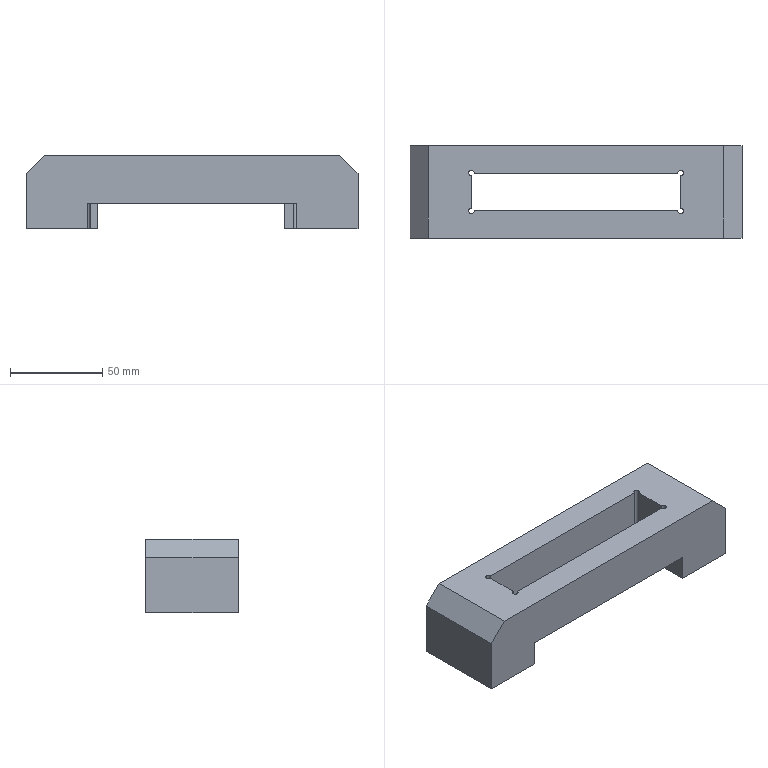Part | SolidWorks | features ICE 3, Chamfer 1, Cut 1, Extrusion 1 | 1 solid | 25 faces | box 180 x 50 x 40 mm | volume 216729 mm3 | plane 19 | cylinder 6 | commonest cylinder face diameters 3 x6
STEP:
#1=CARTESIAN_POINT('',(58.25,-10.25,0.));
#2=VERTEX_POINT('',#1);
#3=CARTESIAN_POINT('',(56.75,-8.75,0.));
#4=VERTEX_POINT('',#3);
#5=CARTESIAN_POINT('',(56.75,-10.25,0.));
#6=DIRECTION('',(0.,0.,1.));
#7=DIRECTION('',(1.,0.,0.));
#8=AXIS2_PLACEMENT_3D('',#5,#6,#7);
#9=CIRCLE('',#8,1.5);
#10=EDGE_CURVE('',#2,#4,#9,.T.);
#11=ORIENTED_EDGE('',*,*,#10,.F.);
#12=CARTESIAN_POINT('',(58.25,-10.25,40.));
#13=VERTEX_POINT('',#12);
#14=CARTESIAN_POINT('',(58.25,-10.25,0.));
#15=DIRECTION('',(0.,0.,1.));
#16=VECTOR('',#15,1000.);
#17=LINE('',#14,#16);
#18=EDGE_CURVE('',#2,#13,#17,.T.);
#19=ORIENTED_EDGE('',*,*,#18,.T.);
#20=CARTESIAN_POINT('',(56.75,-8.75,40.));
#21=VERTEX_POINT('',#20);
#22=CARTESIAN_POINT('',(56.75,-10.25,40.));
#23=DIRECTION('',(0.,0.,1.));
#24=DIRECTION('',(1.,0.,0.));
#25=AXIS2_PLACEMENT_3D('',#22,#23,#24);
#26=CIRCLE('',#25,1.5);
#27=EDGE_CURVE('',#13,#21,#26,.T.);
#28=ORIENTED_EDGE('',*,*,#27,.T.);
#29=CARTESIAN_POINT('',(56.75,-8.75,0.));
#30=DIRECTION('',(0.,0.,1.));
#31=VECTOR('',#30,1000.);
#32=LINE('',#29,#31);
#33=EDGE_CURVE('',#4,#21,#32,.T.);
#34=ORIENTED_EDGE('',*,*,#33,.F.);
#35=EDGE_LOOP('',(#11,#19,#28,#34));
#36=FACE_OUTER_BOUND('',#35,.T.);
#37=CARTESIAN_POINT('',(56.75,-10.25,0.));
#38=DIRECTION('',(0.,0.,1.));
#39=DIRECTION('',(1.,0.,0.));
#40=AXIS2_PLACEMENT_3D('',#37,#38,#39);
#41=CYLINDRICAL_SURFACE('',#40,1.5);
#42=ADVANCED_FACE('',(#36),#41,.F.);
#43=CARTESIAN_POINT('',(58.25,10.25,0.));
#44=VERTEX_POINT('',#43);
#45=CARTESIAN_POINT('',(55.25,10.25,0.));
#46=VERTEX_POINT('',#45);
#47=CARTESIAN_POINT('',(56.75,10.25,0.));
#48=DIRECTION('',(0.,0.,1.));
#49=DIRECTION('',(1.,0.,0.));
#50=AXIS2_PLACEMENT_3D('',#47,#48,#49);
#51=CIRCLE('',#50,1.5);
#52=EDGE_CURVE('',#44,#46,#51,.T.);
#53=ORIENTED_EDGE('',*,*,#52,.F.);
#54=CARTESIAN_POINT('',(58.25,10.25,40.));
#55=VERTEX_POINT('',#54);
#56=CARTESIAN_POINT('',(58.25,10.25,0.));
#57=DIRECTION('',(0.,0.,1.));
#58=VECTOR('',#57,1000.);
#59=LINE('',#56,#58);
#60=EDGE_CURVE('',#44,#55,#59,.T.);
#61=ORIENTED_EDGE('',*,*,#60,.T.);
#62=CARTESIAN_POINT('',(55.25,10.25,40.));
#63=VERTEX_POINT('',#62);
#64=CARTESIAN_POINT('',(56.75,10.25,40.));
#65=DIRECTION('',(0.,0.,1.));
#66=DIRECTION('',(1.,0.,0.));
#67=AXIS2_PLACEMENT_3D('',#64,#65,#66);
#68=CIRCLE('',#67,1.5);
#69=EDGE_CURVE('',#55,#63,#68,.T.);
#70=ORIENTED_EDGE('',*,*,#69,.T.);
#71=CARTESIAN_POINT('',(55.25,10.25,0.));
#72=DIRECTION('',(0.,0.,1.));
#73=VECTOR('',#72,1000.);
#74=LINE('',#71,#73);
#75=EDGE_CURVE('',#46,#63,#74,.T.);
#76=ORIENTED_EDGE('',*,*,#75,.F.);
#77=EDGE_LOOP('',(#53,#61,#70,#76));
#78=FACE_OUTER_BOUND('',#77,.T.);
#79=CARTESIAN_POINT('',(56.75,10.25,0.));
#80=DIRECTION('',(0.,0.,1.));
#81=DIRECTION('',(1.,0.,0.));
#82=AXIS2_PLACEMENT_3D('',#79,#80,#81);
#83=CYLINDRICAL_SURFACE('',#82,1.5);
#84=ADVANCED_FACE('',(#78),#83,.F.);
#85=CARTESIAN_POINT('',(-56.75,-8.75,0.));
#86=VERTEX_POINT('',#85);
#87=CARTESIAN_POINT('',(-56.75,-11.75,0.));
#88=VERTEX_POINT('',#87);
#89=CARTESIAN_POINT('',(-56.75,-10.25,0.));
#90=DIRECTION('',(0.,0.,1.));
#91=DIRECTION('',(1.,0.,0.));
#92=AXIS2_PLACEMENT_3D('',#89,#90,#91);
#93=CIRCLE('',#92,1.5);
#94=EDGE_CURVE('',#86,#88,#93,.T.);
#95=ORIENTED_EDGE('',*,*,#94,.T.);
#96=CARTESIAN_POINT('',(-56.75,-25.,0.));
#97=VERTEX_POINT('',#96);
#98=CARTESIAN_POINT('',(-56.75,-25.,0.));
#99=DIRECTION('',(0.,1.,0.));
#100=VECTOR('',#99,1000.);
#101=LINE('',#98,#100);
#102=EDGE_CURVE('',#97,#88,#101,.T.);
#103=ORIENTED_EDGE('',*,*,#102,.F.);
#104=CARTESIAN_POINT('',(-90.,-25.,0.));
#105=VERTEX_POINT('',#104);
#106=CARTESIAN_POINT('',(-90.,-25.,0.));
#107=DIRECTION('',(1.,0.,0.));
#108=VECTOR('',#107,1000.);
#109=LINE('',#106,#108);
#110=EDGE_CURVE('',#105,#97,#109,.T.);
#111=ORIENTED_EDGE('',*,*,#110,.F.);
#112=CARTESIAN_POINT('',(-90.,25.,0.));
#113=VERTEX_POINT('',#112);
#114=CARTESIAN_POINT('',(-90.,25.,0.));
#115=DIRECTION('',(0.,-1.,0.));
#116=VECTOR('',#115,1000.);
#117=LINE('',#114,#116);
#118=EDGE_CURVE('',#113,#105,#117,.T.);
#119=ORIENTED_EDGE('',*,*,#118,.F.);
#120=CARTESIAN_POINT('',(-51.16,25.,0.));
#121=VERTEX_POINT('',#120);
#122=CARTESIAN_POINT('',(-90.,25.,0.));
#123=DIRECTION('',(-1.,0.,0.));
#124=VECTOR('',#123,1000.);
#125=LINE('',#122,#124);
#126=EDGE_CURVE('',#121,#113,#125,.T.);
#127=ORIENTED_EDGE('',*,*,#126,.F.);
#128=CARTESIAN_POINT('',(-51.16,10.25,0.));
#129=VERTEX_POINT('',#128);
#130=CARTESIAN_POINT('',(-51.16,-5.,0.));
#131=DIRECTION('',(0.,1.,0.));
#132=VECTOR('',#131,1000.);
#133=LINE('',#130,#132);
#134=EDGE_CURVE('',#129,#121,#133,.T.);
#135=ORIENTED_EDGE('',*,*,#134,.F.);
#136=CARTESIAN_POINT('',(-55.25,10.25,0.));
#137=VERTEX_POINT('',#136);
#138=CARTESIAN_POINT('',(-56.75,10.25,0.));
#139=DIRECTION('',(-1.,0.,0.));
#140=VECTOR('',#139,1000.);
#141=LINE('',#138,#140);
#142=EDGE_CURVE('',#129,#137,#141,.T.);
#143=ORIENTED_EDGE('',*,*,#142,.T.);
#144=CARTESIAN_POINT('',(-56.75,8.75,0.));
#145=VERTEX_POINT('',#144);
#146=CARTESIAN_POINT('',(-56.75,10.25,0.));
#147=DIRECTION('',(0.,0.,1.));
#148=DIRECTION('',(1.,0.,0.));
#149=AXIS2_PLACEMENT_3D('',#146,#147,#148);
#150=CIRCLE('',#149,1.5);
#151=EDGE_CURVE('',#137,#145,#150,.T.);
#152=ORIENTED_EDGE('',*,*,#151,.T.);
#153=CARTESIAN_POINT('',(-56.75,10.25,0.));
#154=DIRECTION('',(0.,-1.,0.));
#155=VECTOR('',#154,1000.);
#156=LINE('',#153,#155);
#157=EDGE_CURVE('',#145,#86,#156,.T.);
#158=ORIENTED_EDGE('',*,*,#157,.T.);
#159=EDGE_LOOP('',(#95,#103,#111,#119,#127,#135,#143,#152,#158));
#160=FACE_OUTER_BOUND('',#159,.T.);
#161=CARTESIAN_POINT('',(0.,0.,0.));
#162=DIRECTION('',(0.,0.,1.));
#163=DIRECTION('',(1.,0.,0.));
#164=AXIS2_PLACEMENT_3D('',#161,#162,#163);
#165=PLANE('',#164);
#166=ADVANCED_FACE('',(#160),#165,.F.);
#167=CARTESIAN_POINT('',(-55.25,-10.25,14.));
#168=VERTEX_POINT('',#167);
#169=CARTESIAN_POINT('',(55.25,-10.25,14.));
#170=VERTEX_POINT('',#169);
#171=CARTESIAN_POINT('',(-56.75,-10.25,14.));
#172=DIRECTION('',(1.,0.,0.));
#173=VECTOR('',#172,1000.);
#174=LINE('',#171,#173);
#175=EDGE_CURVE('',#168,#170,#174,.T.);
#176=ORIENTED_EDGE('',*,*,#175,.F.);
#177=CARTESIAN_POINT('',(-55.25,-10.25,40.));
#178=VERTEX_POINT('',#177);
#179=CARTESIAN_POINT('',(-55.25,-10.25,0.));
#180=DIRECTION('',(0.,0.,1.));
#181=VECTOR('',#180,1000.);
#182=LINE('',#179,#181);
#183=EDGE_CURVE('',#168,#178,#182,.T.);
#184=ORIENTED_EDGE('',*,*,#183,.T.);
#185=CARTESIAN_POINT('',(55.25,-10.25,40.));
#186=VERTEX_POINT('',#185);
#187=CARTESIAN_POINT('',(-56.75,-10.25,40.));
#188=DIRECTION('',(1.,0.,0.));
#189=VECTOR('',#188,1000.);
#190=LINE('',#187,#189);
#191=EDGE_CURVE('',#178,#186,#190,.T.);
#192=ORIENTED_EDGE('',*,*,#191,.T.);
#193=CARTESIAN_POINT('',(55.25,-10.25,0.));
#194=DIRECTION('',(0.,0.,-1.));
#195=VECTOR('',#194,1000.);
#196=LINE('',#193,#195);
#197=EDGE_CURVE('',#186,#170,#196,.T.);
#198=ORIENTED_EDGE('',*,*,#197,.T.);
#199=EDGE_LOOP('',(#176,#184,#192,#198));
#200=FACE_OUTER_BOUND('',#199,.T.);
#201=CARTESIAN_POINT('',(-56.75,-10.25,0.));
#202=DIRECTION('',(0.,-1.,0.));
#203=DIRECTION('',(0.,0.,-1.));
#204=AXIS2_PLACEMENT_3D('',#201,#202,#203);
#205=PLANE('',#204);
#206=ADVANCED_FACE('',(#200),#205,.F.);
#207=CARTESIAN_POINT('',(-90.,-25.,30.));
#208=VERTEX_POINT('',#207);
#209=CARTESIAN_POINT('',(-90.,-25.,40.));
#210=DIRECTION('',(0.,0.,-1.));
#211=VECTOR('',#210,1000.);
#212=LINE('',#209,#211);
#213=EDGE_CURVE('',#208,#105,#212,.T.);
#214=ORIENTED_EDGE('',*,*,#213,.F.);
#215=CARTESIAN_POINT('',(-90.,25.,30.));
#216=VERTEX_POINT('',#215);
#217=CARTESIAN_POINT('',(-90.,25.,30.));
#218=DIRECTION('',(0.,1.,0.));
#219=VECTOR('',#218,1000.);
#220=LINE('',#217,#219);
#221=EDGE_CURVE('',#208,#216,#220,.T.);
#222=ORIENTED_EDGE('',*,*,#221,.T.);
#223=CARTESIAN_POINT('',(-90.,25.,40.));
#224=DIRECTION('',(0.,0.,-1.));
#225=VECTOR('',#224,1000.);
#226=LINE('',#223,#225);
#227=EDGE_CURVE('',#216,#113,#226,.T.);
#228=ORIENTED_EDGE('',*,*,#227,.T.);
#229=ORIENTED_EDGE('',*,*,#118,.T.);
#230=EDGE_LOOP('',(#214,#222,#228,#229));
#231=FACE_OUTER_BOUND('',#230,.T.);
#232=CARTESIAN_POINT('',(-90.,25.,40.));
#233=DIRECTION('',(1.,0.,0.));
#234=DIRECTION('',(0.,0.,-1.));
#235=AXIS2_PLACEMENT_3D('',#232,#233,#234);
#236=PLANE('',#235);
#237=ADVANCED_FACE('',(#231),#236,.F.);
#238=CARTESIAN_POINT('',(-80.,-25.,40.));
#239=VERTEX_POINT('',#238);
#240=CARTESIAN_POINT('',(80.,-25.,40.));
#241=VERTEX_POINT('',#240);
#242=CARTESIAN_POINT('',(-90.,-25.,40.));
#243=DIRECTION('',(1.,0.,0.));
#244=VECTOR('',#243,1000.);
#245=LINE('',#242,#244);
#246=EDGE_CURVE('',#239,#241,#245,.T.);
#247=ORIENTED_EDGE('',*,*,#246,.F.);
#248=CARTESIAN_POINT('',(-80.,-25.,40.));
#249=DIRECTION('',(-0.7071,0.,-0.7071));
#250=VECTOR('',#249,1000.);
#251=LINE('',#248,#250);
#252=EDGE_CURVE('',#239,#208,#251,.T.);
#253=ORIENTED_EDGE('',*,*,#252,.T.);
#254=ORIENTED_EDGE('',*,*,#213,.T.);
#255=ORIENTED_EDGE('',*,*,#110,.T.);
#256=CARTESIAN_POINT('',(-56.75,-25.,14.));
#257=VERTEX_POINT('',#256);
#258=CARTESIAN_POINT('',(-56.75,-25.,14.));
#259=DIRECTION('',(0.,0.,-1.));
#260=VECTOR('',#259,1000.);
#261=LINE('',#258,#260);
#262=EDGE_CURVE('',#257,#97,#261,.T.);
#263=ORIENTED_EDGE('',*,*,#262,.F.);
#264=CARTESIAN_POINT('',(56.75,-25.,14.));
#265=VERTEX_POINT('',#264);
#266=CARTESIAN_POINT('',(-56.75,-25.,14.));
#267=DIRECTION('',(-1.,0.,0.));
#268=VECTOR('',#267,1000.);
#269=LINE('',#266,#268);
#270=EDGE_CURVE('',#265,#257,#269,.T.);
#271=ORIENTED_EDGE('',*,*,#270,.F.);
#272=CARTESIAN_POINT('',(56.75,-25.,0.));
#273=VERTEX_POINT('',#272);
#274=CARTESIAN_POINT('',(56.75,-25.,14.));
#275=DIRECTION('',(0.,0.,-1.));
#276=VECTOR('',#275,1000.);
#277=LINE('',#274,#276);
#278=EDGE_CURVE('',#265,#273,#277,.T.);
#279=ORIENTED_EDGE('',*,*,#278,.T.);
#280=CARTESIAN_POINT('',(90.,-25.,0.));
#281=VERTEX_POINT('',#280);
#282=CARTESIAN_POINT('',(-90.,-25.,0.));
#283=DIRECTION('',(1.,0.,0.));
#284=VECTOR('',#283,1000.);
#285=LINE('',#282,#284);
#286=EDGE_CURVE('',#273,#281,#285,.T.);
#287=ORIENTED_EDGE('',*,*,#286,.T.);
#288=CARTESIAN_POINT('',(90.,-25.,30.));
#289=VERTEX_POINT('',#288);
#290=CARTESIAN_POINT('',(90.,-25.,40.));
#291=DIRECTION('',(0.,0.,-1.));
#292=VECTOR('',#291,1000.);
#293=LINE('',#290,#292);
#294=EDGE_CURVE('',#289,#281,#293,.T.);
#295=ORIENTED_EDGE('',*,*,#294,.F.);
#296=CARTESIAN_POINT('',(80.,-25.,40.));
#297=DIRECTION('',(-0.7071,0.,0.7071));
#298=VECTOR('',#297,1000.);
#299=LINE('',#296,#298);
#300=EDGE_CURVE('',#289,#241,#299,.T.);
#301=ORIENTED_EDGE('',*,*,#300,.T.);
#302=EDGE_LOOP('',(#247,#253,#254,#255,#263,#271,#279,#287,#295,#301));
#303=FACE_OUTER_BOUND('',#302,.T.);
#304=CARTESIAN_POINT('',(-90.,-25.,40.));
#305=DIRECTION('',(0.,1.,0.));
#306=DIRECTION('',(0.,0.,1.));
#307=AXIS2_PLACEMENT_3D('',#304,#305,#306);
#308=PLANE('',#307);
#309=ADVANCED_FACE('',(#303),#308,.F.);
#310=CARTESIAN_POINT('',(90.,25.,30.));
#311=VERTEX_POINT('',#310);
#312=CARTESIAN_POINT('',(90.,25.,0.));
#313=VERTEX_POINT('',#312);
#314=CARTESIAN_POINT('',(90.,25.,40.));
#315=DIRECTION('',(0.,0.,-1.));
#316=VECTOR('',#315,1000.);
#317=LINE('',#314,#316);
#318=EDGE_CURVE('',#311,#313,#317,.T.);
#319=ORIENTED_EDGE('',*,*,#318,.F.);
#320=CARTESIAN_POINT('',(90.,-25.,30.));
#321=DIRECTION('',(0.,-1.,0.));
#322=VECTOR('',#321,1000.);
#323=LINE('',#320,#322);
#324=EDGE_CURVE('',#311,#289,#323,.T.);
#325=ORIENTED_EDGE('',*,*,#324,.T.);
#326=ORIENTED_EDGE('',*,*,#294,.T.);
#327=CARTESIAN_POINT('',(90.,25.,0.));
#328=DIRECTION('',(0.,1.,0.));
#329=VECTOR('',#328,1000.);
#330=LINE('',#327,#329);
#331=EDGE_CURVE('',#281,#313,#330,.T.);
#332=ORIENTED_EDGE('',*,*,#331,.T.);
#333=EDGE_LOOP('',(#319,#325,#326,#332));
#334=FACE_OUTER_BOUND('',#333,.T.);
#335=CARTESIAN_POINT('',(90.,25.,40.));
#336=DIRECTION('',(-1.,0.,0.));
#337=DIRECTION('',(0.,0.,1.));
#338=AXIS2_PLACEMENT_3D('',#335,#336,#337);
#339=PLANE('',#338);
#340=ADVANCED_FACE('',(#334),#339,.F.);
#341=ORIENTED_EDGE('',*,*,#227,.F.);
#342=CARTESIAN_POINT('',(-80.,25.,40.));
#343=VERTEX_POINT('',#342);
#344=CARTESIAN_POINT('',(-80.,25.,40.));
#345=DIRECTION('',(0.7071,0.,0.7071));
#346=VECTOR('',#345,1000.);
#347=LINE('',#344,#346);
#348=EDGE_CURVE('',#216,#343,#347,.T.);
#349=ORIENTED_EDGE('',*,*,#348,.T.);
#350=CARTESIAN_POINT('',(80.,25.,40.));
#351=VERTEX_POINT('',#350);
#352=CARTESIAN_POINT('',(-90.,25.,40.));
#353=DIRECTION('',(-1.,0.,0.));
#354=VECTOR('',#353,1000.);
#355=LINE('',#352,#354);
#356=EDGE_CURVE('',#351,#343,#355,.T.);
#357=ORIENTED_EDGE('',*,*,#356,.F.);
#358=CARTESIAN_POINT('',(80.,25.,40.));
#359=DIRECTION('',(0.7071,0.,-0.7071));
#360=VECTOR('',#359,1000.);
#361=LINE('',#358,#360);
#362=EDGE_CURVE('',#351,#311,#361,.T.);
#363=ORIENTED_EDGE('',*,*,#362,.T.);
#364=ORIENTED_EDGE('',*,*,#318,.T.);
#365=CARTESIAN_POINT('',(50.364,25.,0.));
#366=VERTEX_POINT('',#365);
#367=CARTESIAN_POINT('',(-90.,25.,0.));
#368=DIRECTION('',(-1.,0.,0.));
#369=VECTOR('',#368,1000.);
#370=LINE('',#367,#369);
#371=EDGE_CURVE('',#313,#366,#370,.T.);
#372=ORIENTED_EDGE('',*,*,#371,.T.);
#373=CARTESIAN_POINT('',(50.364,25.,14.));
#374=VERTEX_POINT('',#373);
#375=CARTESIAN_POINT('',(50.364,25.,0.));
#376=DIRECTION('',(0.,0.,-1.));
#377=VECTOR('',#376,1000.);
#378=LINE('',#375,#377);
#379=EDGE_CURVE('',#374,#366,#378,.T.);
#380=ORIENTED_EDGE('',*,*,#379,.F.);
#381=CARTESIAN_POINT('',(-51.16,25.,14.));
#382=VERTEX_POINT('',#381);
#383=CARTESIAN_POINT('',(50.364,25.,14.));
#384=DIRECTION('',(1.,0.,0.));
#385=VECTOR('',#384,1000.);
#386=LINE('',#383,#385);
#387=EDGE_CURVE('',#382,#374,#386,.T.);
#388=ORIENTED_EDGE('',*,*,#387,.F.);
#389=CARTESIAN_POINT('',(-51.16,25.,0.));
#390=DIRECTION('',(0.,0.,1.));
#391=VECTOR('',#390,1000.);
#392=LINE('',#389,#391);
#393=EDGE_CURVE('',#121,#382,#392,.T.);
#394=ORIENTED_EDGE('',*,*,#393,.F.);
#395=ORIENTED_EDGE('',*,*,#126,.T.);
#396=EDGE_LOOP('',(#341,#349,#357,#363,#364,#372,#380,#388,#394,#395));
#397=FACE_OUTER_BOUND('',#396,.T.);
#398=CARTESIAN_POINT('',(-90.,25.,40.));
#399=DIRECTION('',(0.,-1.,0.));
#400=DIRECTION('',(0.,0.,-1.));
#401=AXIS2_PLACEMENT_3D('',#398,#399,#400);
#402=PLANE('',#401);
#403=ADVANCED_FACE('',(#397),#402,.F.);
#404=CARTESIAN_POINT('',(56.75,-10.25,40.));
#405=DIRECTION('',(0.,0.,1.));
#406=DIRECTION('',(1.,0.,0.));
#407=AXIS2_PLACEMENT_3D('',#404,#405,#406);
#408=CIRCLE('',#407,1.5);
#409=EDGE_CURVE('',#186,#13,#408,.T.);
#410=ORIENTED_EDGE('',*,*,#409,.F.);
#411=ORIENTED_EDGE('',*,*,#191,.F.);
#412=CARTESIAN_POINT('',(-56.75,-8.75,40.));
#413=VERTEX_POINT('',#412);
#414=CARTESIAN_POINT('',(-56.75,-10.25,40.));
#415=DIRECTION('',(0.,0.,1.));
#416=DIRECTION('',(1.,0.,0.));
#417=AXIS2_PLACEMENT_3D('',#414,#415,#416);
#418=CIRCLE('',#417,1.5);
#419=EDGE_CURVE('',#413,#178,#418,.T.);
#420=ORIENTED_EDGE('',*,*,#419,.F.);
#421=CARTESIAN_POINT('',(-56.75,8.75,40.));
#422=VERTEX_POINT('',#421);
#423=CARTESIAN_POINT('',(-56.75,10.25,40.));
#424=DIRECTION('',(0.,-1.,0.));
#425=VECTOR('',#424,1000.);
#426=LINE('',#423,#425);
#427=EDGE_CURVE('',#422,#413,#426,.T.);
#428=ORIENTED_EDGE('',*,*,#427,.F.);
#429=CARTESIAN_POINT('',(-55.25,10.25,40.));
#430=VERTEX_POINT('',#429);
#431=CARTESIAN_POINT('',(-56.75,10.25,40.));
#432=DIRECTION('',(0.,0.,1.));
#433=DIRECTION('',(1.,0.,0.));
#434=AXIS2_PLACEMENT_3D('',#431,#432,#433);
#435=CIRCLE('',#434,1.5);
#436=EDGE_CURVE('',#430,#422,#435,.T.);
#437=ORIENTED_EDGE('',*,*,#436,.F.);
#438=CARTESIAN_POINT('',(-56.75,10.25,40.));
#439=DIRECTION('',(-1.,0.,0.));
#440=VECTOR('',#439,1000.);
#441=LINE('',#438,#440);
#442=EDGE_CURVE('',#63,#430,#441,.T.);
#443=ORIENTED_EDGE('',*,*,#442,.F.);
#444=ORIENTED_EDGE('',*,*,#69,.F.);
#445=CARTESIAN_POINT('',(56.75,8.75,40.));
#446=VERTEX_POINT('',#445);
#447=CARTESIAN_POINT('',(56.75,10.25,40.));
#448=DIRECTION('',(0.,0.,1.));
#449=DIRECTION('',(1.,0.,0.));
#450=AXIS2_PLACEMENT_3D('',#447,#448,#449);
#451=CIRCLE('',#450,1.5);
#452=EDGE_CURVE('',#446,#55,#451,.T.);
#453=ORIENTED_EDGE('',*,*,#452,.F.);
#454=CARTESIAN_POINT('',(56.75,10.25,40.));
#455=DIRECTION('',(0.,1.,0.));
#456=VECTOR('',#455,1000.);
#457=LINE('',#454,#456);
#458=EDGE_CURVE('',#21,#446,#457,.T.);
#459=ORIENTED_EDGE('',*,*,#458,.F.);
#460=ORIENTED_EDGE('',*,*,#27,.F.);
#461=EDGE_LOOP('',(#410,#411,#420,#428,#437,#443,#444,#453,#459,#460));
#462=FACE_BOUND('',#461,.T.);
#463=ORIENTED_EDGE('',*,*,#356,.T.);
#464=CARTESIAN_POINT('',(-80.,-25.,40.));
#465=DIRECTION('',(0.,-1.,0.));
#466=VECTOR('',#465,1000.);
#467=LINE('',#464,#466);
#468=EDGE_CURVE('',#343,#239,#467,.T.);
#469=ORIENTED_EDGE('',*,*,#468,.T.);
#470=ORIENTED_EDGE('',*,*,#246,.T.);
#471=CARTESIAN_POINT('',(80.,25.,40.));
#472=DIRECTION('',(0.,1.,0.));
#473=VECTOR('',#472,1000.);
#474=LINE('',#471,#473);
#475=EDGE_CURVE('',#241,#351,#474,.T.);
#476=ORIENTED_EDGE('',*,*,#475,.T.);
#477=EDGE_LOOP('',(#463,#469,#470,#476));
#478=FACE_OUTER_BOUND('',#477,.T.);
#479=CARTESIAN_POINT('',(0.,0.,40.));
#480=DIRECTION('',(0.,0.,1.));
#481=DIRECTION('',(1.,0.,0.));
#482=AXIS2_PLACEMENT_3D('',#479,#480,#481);
#483=PLANE('',#482);
#484=ADVANCED_FACE('',(#462,#478),#483,.T.);
#485=ORIENTED_EDGE('',*,*,#286,.F.);
#486=CARTESIAN_POINT('',(56.75,-11.75,0.));
#487=VERTEX_POINT('',#486);
#488=CARTESIAN_POINT('',(56.75,-25.,0.));
#489=DIRECTION('',(0.,-1.,0.));
#490=VECTOR('',#489,1000.);
#491=LINE('',#488,#490);
#492=EDGE_CURVE('',#487,#273,#491,.T.);
#493=ORIENTED_EDGE('',*,*,#492,.F.);
#494=CARTESIAN_POINT('',(56.75,-10.25,0.));
#495=DIRECTION('',(0.,0.,1.));
#496=DIRECTION('',(1.,0.,0.));
#497=AXIS2_PLACEMENT_3D('',#494,#495,#496);
#498=CIRCLE('',#497,1.5);
#499=EDGE_CURVE('',#487,#2,#498,.T.);
#500=ORIENTED_EDGE('',*,*,#499,.T.);
#501=ORIENTED_EDGE('',*,*,#10,.T.);
#502=CARTESIAN_POINT('',(56.75,8.75,0.));
#503=VERTEX_POINT('',#502);
#504=CARTESIAN_POINT('',(56.75,10.25,0.));
#505=DIRECTION('',(0.,1.,0.));
#506=VECTOR('',#505,1000.);
#507=LINE('',#504,#506);
#508=EDGE_CURVE('',#4,#503,#507,.T.);
#509=ORIENTED_EDGE('',*,*,#508,.T.);
#510=CARTESIAN_POINT('',(56.75,10.25,0.));
#511=DIRECTION('',(0.,0.,1.));
#512=DIRECTION('',(1.,0.,0.));
#513=AXIS2_PLACEMENT_3D('',#510,#511,#512);
#514=CIRCLE('',#513,1.5);
#515=EDGE_CURVE('',#503,#44,#514,.T.);
#516=ORIENTED_EDGE('',*,*,#515,.T.);
#517=ORIENTED_EDGE('',*,*,#52,.T.);
#518=CARTESIAN_POINT('',(50.364,10.25,0.));
#519=VERTEX_POINT('',#518);
#520=CARTESIAN_POINT('',(-56.75,10.25,0.));
#521=DIRECTION('',(-1.,0.,0.));
#522=VECTOR('',#521,1000.);
#523=LINE('',#520,#522);
#524=EDGE_CURVE('',#46,#519,#523,.T.);
#525=ORIENTED_EDGE('',*,*,#524,.T.);
#526=CARTESIAN_POINT('',(50.364,-5.,0.));
#527=DIRECTION('',(0.,1.,0.));
#528=VECTOR('',#527,1000.);
#529=LINE('',#526,#528);
#530=EDGE_CURVE('',#519,#366,#529,.T.);
#531=ORIENTED_EDGE('',*,*,#530,.T.);
#532=ORIENTED_EDGE('',*,*,#371,.F.);
#533=ORIENTED_EDGE('',*,*,#331,.F.);
#534=EDGE_LOOP('',(#485,#493,#500,#501,#509,#516,#517,#525,#531,#532,#533));
#535=FACE_OUTER_BOUND('',#534,.T.);
#536=CARTESIAN_POINT('',(0.,0.,0.));
#537=DIRECTION('',(0.,0.,1.));
#538=DIRECTION('',(1.,0.,0.));
#539=AXIS2_PLACEMENT_3D('',#536,#537,#538);
#540=PLANE('',#539);
#541=ADVANCED_FACE('',(#535),#540,.F.);
#542=ORIENTED_EDGE('',*,*,#508,.F.);
#543=ORIENTED_EDGE('',*,*,#33,.T.);
#544=ORIENTED_EDGE('',*,*,#458,.T.);
#545=CARTESIAN_POINT('',(56.75,8.75,0.));
#546=DIRECTION('',(0.,0.,-1.));
#547=VECTOR('',#546,1000.);
#548=LINE('',#545,#547);
#549=EDGE_CURVE('',#446,#503,#548,.T.);
#550=ORIENTED_EDGE('',*,*,#549,.T.);
#551=EDGE_LOOP('',(#542,#543,#544,#550));
#552=FACE_OUTER_BOUND('',#551,.T.);
#553=CARTESIAN_POINT('',(56.75,10.25,0.));
#554=DIRECTION('',(1.,0.,0.));
#555=DIRECTION('',(0.,0.,-1.));
#556=AXIS2_PLACEMENT_3D('',#553,#554,#555);
#557=PLANE('',#556);
#558=ADVANCED_FACE('',(#552),#557,.F.);
#559=ORIENTED_EDGE('',*,*,#427,.T.);
#560=CARTESIAN_POINT('',(-56.75,-8.75,0.));
#561=DIRECTION('',(0.,0.,-1.));
#562=VECTOR('',#561,1000.);
#563=LINE('',#560,#562);
#564=EDGE_CURVE('',#413,#86,#563,.T.);
#565=ORIENTED_EDGE('',*,*,#564,.T.);
#566=ORIENTED_EDGE('',*,*,#157,.F.);
#567=CARTESIAN_POINT('',(-56.75,8.75,0.));
#568=DIRECTION('',(0.,0.,1.));
#569=VECTOR('',#568,1000.);
#570=LINE('',#567,#569);
#571=EDGE_CURVE('',#145,#422,#570,.T.);
#572=ORIENTED_EDGE('',*,*,#571,.T.);
#573=EDGE_LOOP('',(#559,#565,#566,#572));
#574=FACE_OUTER_BOUND('',#573,.T.);
#575=CARTESIAN_POINT('',(-56.75,10.25,0.));
#576=DIRECTION('',(-1.,0.,0.));
#577=DIRECTION('',(0.,0.,1.));
#578=AXIS2_PLACEMENT_3D('',#575,#576,#577);
#579=PLANE('',#578);
#580=ADVANCED_FACE('',(#574),#579,.F.);
#581=CARTESIAN_POINT('',(-51.16,10.25,14.));
#582=VERTEX_POINT('',#581);
#583=CARTESIAN_POINT('',(50.364,10.25,14.));
#584=VERTEX_POINT('',#583);
#585=CARTESIAN_POINT('',(-56.75,10.25,14.));
#586=DIRECTION('',(1.,0.,0.));
#587=VECTOR('',#586,1000.);
#588=LINE('',#585,#587);
#589=EDGE_CURVE('',#582,#584,#588,.T.);
#590=ORIENTED_EDGE('',*,*,#589,.T.);
#591=CARTESIAN_POINT('',(50.364,10.25,0.));
#592=DIRECTION('',(0.,0.,-1.));
#593=VECTOR('',#592,1000.);
#594=LINE('',#591,#593);
#595=EDGE_CURVE('',#584,#519,#594,.T.);
#596=ORIENTED_EDGE('',*,*,#595,.T.);
#597=ORIENTED_EDGE('',*,*,#524,.F.);
#598=ORIENTED_EDGE('',*,*,#75,.T.);
#599=ORIENTED_EDGE('',*,*,#442,.T.);
#600=CARTESIAN_POINT('',(-55.25,10.25,0.));
#601=DIRECTION('',(0.,0.,-1.));
#602=VECTOR('',#601,1000.);
#603=LINE('',#600,#602);
#604=EDGE_CURVE('',#430,#137,#603,.T.);
#605=ORIENTED_EDGE('',*,*,#604,.T.);
#606=ORIENTED_EDGE('',*,*,#142,.F.);
#607=CARTESIAN_POINT('',(-51.16,10.25,0.));
#608=DIRECTION('',(0.,0.,1.));
#609=VECTOR('',#608,1000.);
#610=LINE('',#607,#609);
#611=EDGE_CURVE('',#129,#582,#610,.T.);
#612=ORIENTED_EDGE('',*,*,#611,.T.);
#613=EDGE_LOOP('',(#590,#596,#597,#598,#599,#605,#606,#612));
#614=FACE_OUTER_BOUND('',#613,.T.);
#615=CARTESIAN_POINT('',(-56.75,10.25,0.));
#616=DIRECTION('',(0.,1.,0.));
#617=DIRECTION('',(0.,0.,1.));
#618=AXIS2_PLACEMENT_3D('',#615,#616,#617);
#619=PLANE('',#618);
#620=ADVANCED_FACE('',(#614),#619,.F.);
#621=ORIENTED_EDGE('',*,*,#151,.F.);
#622=ORIENTED_EDGE('',*,*,#604,.F.);
#623=ORIENTED_EDGE('',*,*,#436,.T.);
#624=ORIENTED_EDGE('',*,*,#571,.F.);
#625=EDGE_LOOP('',(#621,#622,#623,#624));
#626=FACE_OUTER_BOUND('',#625,.T.);
#627=CARTESIAN_POINT('',(-56.75,10.25,0.));
#628=DIRECTION('',(0.,0.,1.));
#629=DIRECTION('',(1.,0.,0.));
#630=AXIS2_PLACEMENT_3D('',#627,#628,#629);
#631=CYLINDRICAL_SURFACE('',#630,1.5);
#632=ADVANCED_FACE('',(#626),#631,.F.);
#633=CARTESIAN_POINT('',(-56.75,-11.75,14.));
#634=VERTEX_POINT('',#633);
#635=CARTESIAN_POINT('',(-56.75,-10.25,14.));
#636=DIRECTION('',(0.,0.,1.));
#637=DIRECTION('',(-1.,0.,0.));
#638=AXIS2_PLACEMENT_3D('',#635,#636,#637);
#639=CIRCLE('',#638,1.5);
#640=EDGE_CURVE('',#634,#168,#639,.T.);
#641=ORIENTED_EDGE('',*,*,#640,.F.);
#642=CARTESIAN_POINT('',(-56.75,-11.75,0.));
#643=DIRECTION('',(0.,0.,-1.));
#644=VECTOR('',#643,1000.);
#645=LINE('',#642,#644);
#646=EDGE_CURVE('',#634,#88,#645,.T.);
#647=ORIENTED_EDGE('',*,*,#646,.T.);
#648=ORIENTED_EDGE('',*,*,#94,.F.);
#649=ORIENTED_EDGE('',*,*,#564,.F.);
#650=ORIENTED_EDGE('',*,*,#419,.T.);
#651=ORIENTED_EDGE('',*,*,#183,.F.);
#652=EDGE_LOOP('',(#641,#647,#648,#649,#650,#651));
#653=FACE_OUTER_BOUND('',#652,.T.);
#654=CARTESIAN_POINT('',(-56.75,-10.25,0.));
#655=DIRECTION('',(0.,0.,1.));
#656=DIRECTION('',(1.,0.,0.));
#657=AXIS2_PLACEMENT_3D('',#654,#655,#656);
#658=CYLINDRICAL_SURFACE('',#657,1.5);
#659=ADVANCED_FACE('',(#653),#658,.F.);
#660=ORIENTED_EDGE('',*,*,#60,.F.);
#661=ORIENTED_EDGE('',*,*,#515,.F.);
#662=ORIENTED_EDGE('',*,*,#549,.F.);
#663=ORIENTED_EDGE('',*,*,#452,.T.);
#664=EDGE_LOOP('',(#660,#661,#662,#663));
#665=FACE_OUTER_BOUND('',#664,.T.);
#666=CARTESIAN_POINT('',(56.75,10.25,0.));
#667=DIRECTION('',(0.,0.,1.));
#668=DIRECTION('',(1.,0.,0.));
#669=AXIS2_PLACEMENT_3D('',#666,#667,#668);
#670=CYLINDRICAL_SURFACE('',#669,1.5);
#671=ADVANCED_FACE('',(#665),#670,.F.);
#672=ORIENTED_EDGE('',*,*,#18,.F.);
#673=ORIENTED_EDGE('',*,*,#499,.F.);
#674=CARTESIAN_POINT('',(56.75,-11.75,14.));
#675=VERTEX_POINT('',#674);
#676=CARTESIAN_POINT('',(56.75,-11.75,0.));
#677=DIRECTION('',(0.,0.,1.));
#678=VECTOR('',#677,1000.);
#679=LINE('',#676,#678);
#680=EDGE_CURVE('',#487,#675,#679,.T.);
#681=ORIENTED_EDGE('',*,*,#680,.T.);
#682=CARTESIAN_POINT('',(56.75,-10.25,14.));
#683=DIRECTION('',(0.,0.,1.));
#684=DIRECTION('',(-1.,0.,0.));
#685=AXIS2_PLACEMENT_3D('',#682,#683,#684);
#686=CIRCLE('',#685,1.5);
#687=EDGE_CURVE('',#170,#675,#686,.T.);
#688=ORIENTED_EDGE('',*,*,#687,.F.);
#689=ORIENTED_EDGE('',*,*,#197,.F.);
#690=ORIENTED_EDGE('',*,*,#409,.T.);
#691=EDGE_LOOP('',(#672,#673,#681,#688,#689,#690));
#692=FACE_OUTER_BOUND('',#691,.T.);
#693=CARTESIAN_POINT('',(56.75,-10.25,0.));
#694=DIRECTION('',(0.,0.,1.));
#695=DIRECTION('',(1.,0.,0.));
#696=AXIS2_PLACEMENT_3D('',#693,#694,#695);
#697=CYLINDRICAL_SURFACE('',#696,1.5);
#698=ADVANCED_FACE('',(#692),#697,.F.);
#699=CARTESIAN_POINT('',(50.364,-5.,14.));
#700=DIRECTION('',(0.,1.,0.));
#701=VECTOR('',#700,1000.);
#702=LINE('',#699,#701);
#703=EDGE_CURVE('',#584,#374,#702,.T.);
#704=ORIENTED_EDGE('',*,*,#703,.T.);
#705=ORIENTED_EDGE('',*,*,#379,.T.);
#706=ORIENTED_EDGE('',*,*,#530,.F.);
#707=ORIENTED_EDGE('',*,*,#595,.F.);
#708=EDGE_LOOP('',(#704,#705,#706,#707));
#709=FACE_OUTER_BOUND('',#708,.T.);
#710=CARTESIAN_POINT('',(50.364,-5.,0.));
#711=DIRECTION('',(1.,0.,0.));
#712=DIRECTION('',(0.,0.,-1.));
#713=AXIS2_PLACEMENT_3D('',#710,#711,#712);
#714=PLANE('',#713);
#715=ADVANCED_FACE('',(#709),#714,.F.);
#716=CARTESIAN_POINT('',(-51.16,-5.,14.));
#717=DIRECTION('',(0.,1.,0.));
#718=VECTOR('',#717,1000.);
#719=LINE('',#716,#718);
#720=EDGE_CURVE('',#582,#382,#719,.T.);
#721=ORIENTED_EDGE('',*,*,#720,.T.);
#722=ORIENTED_EDGE('',*,*,#387,.T.);
#723=ORIENTED_EDGE('',*,*,#703,.F.);
#724=ORIENTED_EDGE('',*,*,#589,.F.);
#725=EDGE_LOOP('',(#721,#722,#723,#724));
#726=FACE_OUTER_BOUND('',#725,.T.);
#727=CARTESIAN_POINT('',(50.364,-5.,14.));
#728=DIRECTION('',(0.,0.,1.));
#729=DIRECTION('',(1.,0.,0.));
#730=AXIS2_PLACEMENT_3D('',#727,#728,#729);
#731=PLANE('',#730);
#732=ADVANCED_FACE('',(#726),#731,.F.);
#733=ORIENTED_EDGE('',*,*,#134,.T.);
#734=ORIENTED_EDGE('',*,*,#393,.T.);
#735=ORIENTED_EDGE('',*,*,#720,.F.);
#736=ORIENTED_EDGE('',*,*,#611,.F.);
#737=EDGE_LOOP('',(#733,#734,#735,#736));
#738=FACE_OUTER_BOUND('',#737,.T.);
#739=CARTESIAN_POINT('',(-51.16,-5.,0.));
#740=DIRECTION('',(-1.,0.,0.));
#741=DIRECTION('',(0.,0.,1.));
#742=AXIS2_PLACEMENT_3D('',#739,#740,#741);
#743=PLANE('',#742);
#744=ADVANCED_FACE('',(#738),#743,.F.);
#745=CARTESIAN_POINT('',(-56.75,-25.,14.));
#746=DIRECTION('',(0.,1.,0.));
#747=VECTOR('',#746,1000.);
#748=LINE('',#745,#747);
#749=EDGE_CURVE('',#257,#634,#748,.T.);
#750=ORIENTED_EDGE('',*,*,#749,.F.);
#751=ORIENTED_EDGE('',*,*,#262,.T.);
#752=ORIENTED_EDGE('',*,*,#102,.T.);
#753=ORIENTED_EDGE('',*,*,#646,.F.);
#754=EDGE_LOOP('',(#750,#751,#752,#753));
#755=FACE_OUTER_BOUND('',#754,.T.);
#756=CARTESIAN_POINT('',(-56.75,-25.,14.));
#757=DIRECTION('',(-1.,0.,0.));
#758=DIRECTION('',(0.,0.,1.));
#759=AXIS2_PLACEMENT_3D('',#756,#757,#758);
#760=PLANE('',#759);
#761=ADVANCED_FACE('',(#755),#760,.F.);
#762=ORIENTED_EDGE('',*,*,#492,.T.);
#763=ORIENTED_EDGE('',*,*,#278,.F.);
#764=CARTESIAN_POINT('',(56.75,-25.,14.));
#765=DIRECTION('',(0.,-1.,0.));
#766=VECTOR('',#765,1000.);
#767=LINE('',#764,#766);
#768=EDGE_CURVE('',#675,#265,#767,.T.);
#769=ORIENTED_EDGE('',*,*,#768,.F.);
#770=ORIENTED_EDGE('',*,*,#680,.F.);
#771=EDGE_LOOP('',(#762,#763,#769,#770));
#772=FACE_OUTER_BOUND('',#771,.T.);
#773=CARTESIAN_POINT('',(56.75,-25.,14.));
#774=DIRECTION('',(1.,0.,0.));
#775=DIRECTION('',(0.,0.,-1.));
#776=AXIS2_PLACEMENT_3D('',#773,#774,#775);
#777=PLANE('',#776);
#778=ADVANCED_FACE('',(#772),#777,.F.);
#779=ORIENTED_EDGE('',*,*,#640,.T.);
#780=ORIENTED_EDGE('',*,*,#175,.T.);
#781=ORIENTED_EDGE('',*,*,#687,.T.);
#782=ORIENTED_EDGE('',*,*,#768,.T.);
#783=ORIENTED_EDGE('',*,*,#270,.T.);
#784=ORIENTED_EDGE('',*,*,#749,.T.);
#785=EDGE_LOOP('',(#779,#780,#781,#782,#783,#784));
#786=FACE_OUTER_BOUND('',#785,.T.);
#787=CARTESIAN_POINT('',(0.,0.,14.));
#788=DIRECTION('',(0.,0.,-1.));
#789=DIRECTION('',(-1.,0.,0.));
#790=AXIS2_PLACEMENT_3D('',#787,#788,#789);
#791=PLANE('',#790);
#792=ADVANCED_FACE('',(#786),#791,.T.);
#793=ORIENTED_EDGE('',*,*,#348,.F.);
#794=ORIENTED_EDGE('',*,*,#221,.F.);
#795=ORIENTED_EDGE('',*,*,#252,.F.);
#796=ORIENTED_EDGE('',*,*,#468,.F.);
#797=EDGE_LOOP('',(#793,#794,#795,#796));
#798=FACE_OUTER_BOUND('',#797,.T.);
#799=CARTESIAN_POINT('',(-80.,0.,40.));
#800=DIRECTION('',(-0.7071,0.,0.7071));
#801=DIRECTION('',(0.,1.,0.));
#802=AXIS2_PLACEMENT_3D('',#799,#800,#801);
#803=PLANE('',#802);
#804=ADVANCED_FACE('',(#798),#803,.T.);
#805=ORIENTED_EDGE('',*,*,#300,.F.);
#806=ORIENTED_EDGE('',*,*,#324,.F.);
#807=ORIENTED_EDGE('',*,*,#362,.F.);
#808=ORIENTED_EDGE('',*,*,#475,.F.);
#809=EDGE_LOOP('',(#805,#806,#807,#808));
#810=FACE_OUTER_BOUND('',#809,.T.);
#811=CARTESIAN_POINT('',(80.,0.,40.));
#812=DIRECTION('',(0.7071,0.,0.7071));
#813=DIRECTION('',(0.,-1.,0.));
#814=AXIS2_PLACEMENT_3D('',#811,#812,#813);
#815=PLANE('',#814);
#816=ADVANCED_FACE('',(#810),#815,.T.);
#817=CLOSED_SHELL('',(#42,#84,#166,#206,#237,#309,#340,#403,#484,#541,#558,#580,#620,#632,#659,#671,#698,#715,#732,#744,#761,#778,#792,#804,#816));
#818=MANIFOLD_SOLID_BREP('',#817);
#819=CARTESIAN_POINT('',(0.,0.,0.));
#820=DIRECTION('',(0.,0.,1.));
#821=DIRECTION('',(1.,0.,0.));
#822=AXIS2_PLACEMENT_3D('',#819,#820,#821);
#823=(LENGTH_UNIT()NAMED_UNIT(*)SI_UNIT(.MILLI.,.METRE.));
#824=UNCERTAINTY_MEASURE_WITH_UNIT(LENGTH_MEASURE(0.00001),#823,'','');
#825=(NAMED_UNIT(*)PLANE_ANGLE_UNIT()SI_UNIT($,.RADIAN.));
#826=(NAMED_UNIT(*)SI_UNIT($,.STERADIAN.)SOLID_ANGLE_UNIT());
#827=(GEOMETRIC_REPRESENTATION_CONTEXT(3)GLOBAL_UNCERTAINTY_ASSIGNED_CONTEXT((#824))GLOBAL_UNIT_ASSIGNED_CONTEXT((#823,#825,#826))REPRESENTATION_CONTEXT('',''));
#828=ADVANCED_BREP_SHAPE_REPRESENTATION('',(#818,#822),#827);